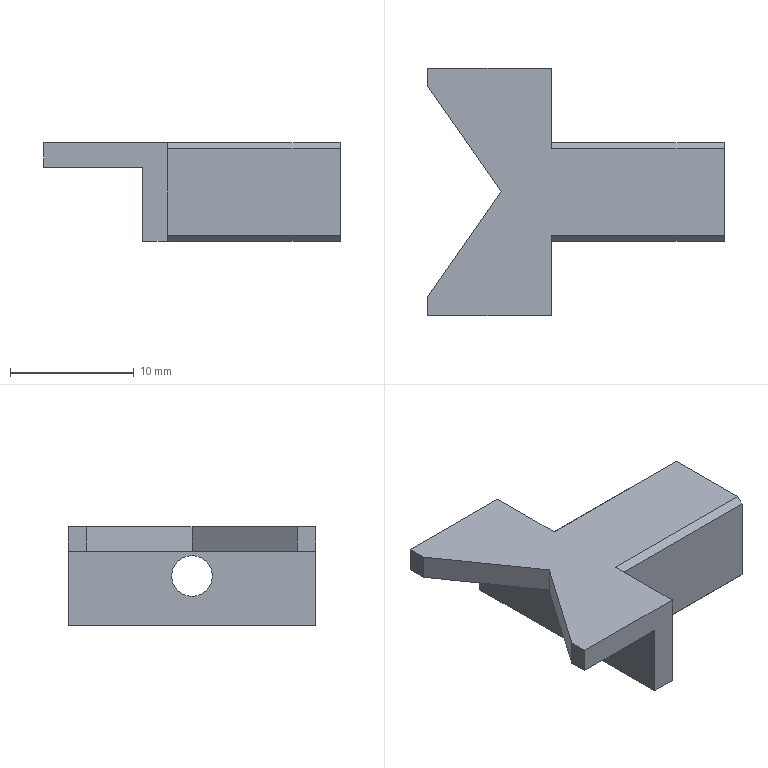Part | STEP file | PN_0017 | 1 solid | 21 faces | box 24 x 20 x 8 mm | volume 1291 mm3 | plane 19 | cylinder 2 | commonest cylinder face diameters 3.3 x2